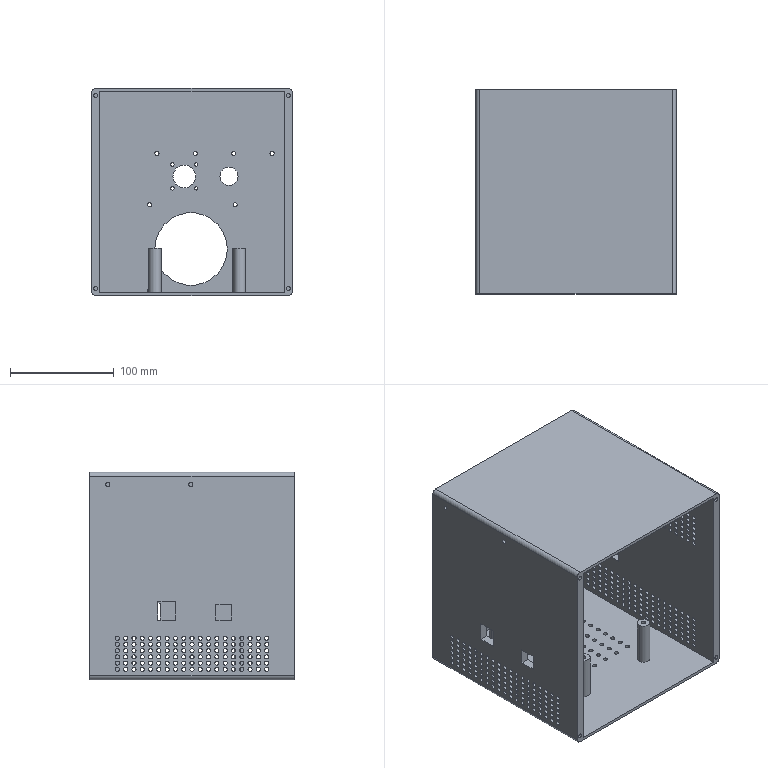Part | SolidWorks | features ICE 18, OffsetRefSurface 2, Thicken 2, BossThin 1, Chamfer 1, Extrusion 1, Fillet 1, LPattern 1, MirrorPattern 1, Shell 1 | 1 solid | 915 faces | box 193.595 x 197 x 200 mm | volume 952035 mm3 | cylinder 866 | plane 41 | cone 8 | commonest cylinder face diameters 4 x832 8 x12 3.2 x8 12 x8 17.5 x2 22 x2